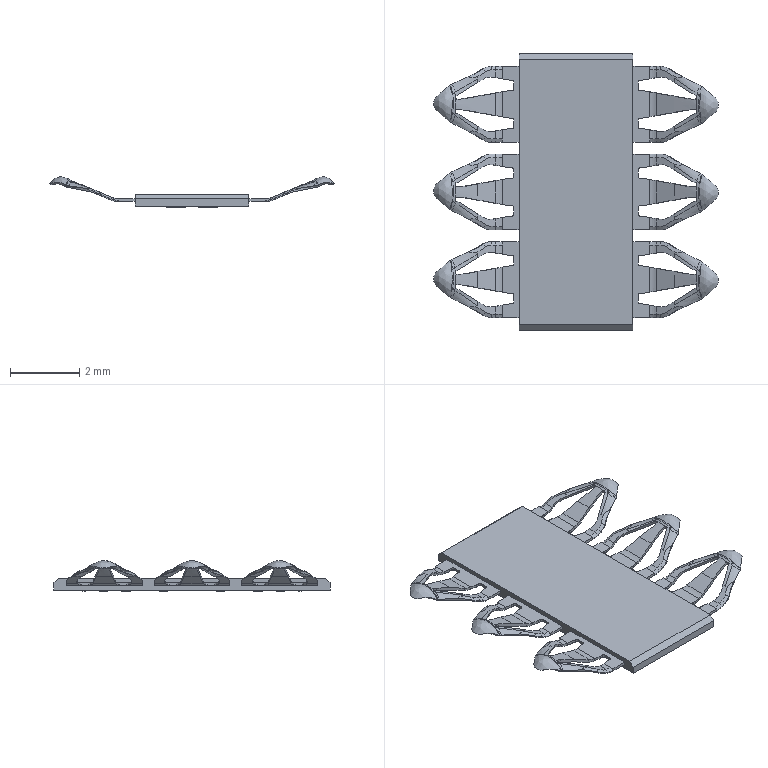Part | Creo | 1 solid | 622 faces | box 8.25 x 8 x 0.8796 mm | volume 10.592 mm3 | plane 260 | spline 180 | cylinder 158 | cone 24 | commonest cylinder face diameters 1 x78 0.1 x44 1.16 x18 0.2 x12 0.36 x6